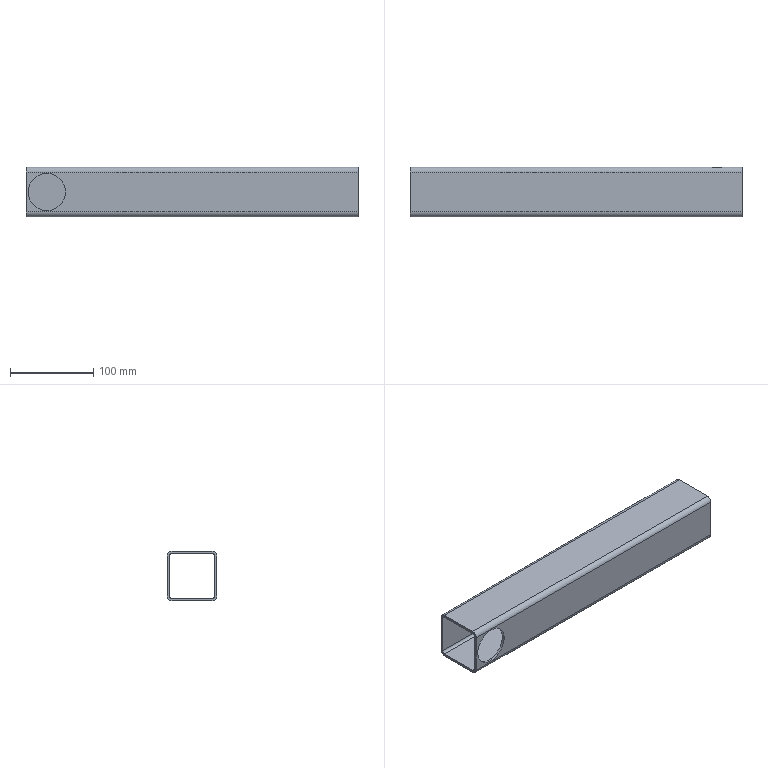Part | STEP file | JBJ-P-1016-02_Default<As Machined> | 1 solid | 24 faces | box 400 x 60 x 60 mm | volume 252664 mm3 | plane 12 | cylinder 12 | commonest cylinder face diameters 6 x6 12 x4 45 x1 54 x1
STEP:
#1=CARTESIAN_POINT('',(400.,30.,-24.));
#2=VERTEX_POINT('',#1);
#3=CARTESIAN_POINT('',(382.369,30.,-24.));
#4=VERTEX_POINT('',#3);
#5=CARTESIAN_POINT('',(400.,30.,-24.));
#6=DIRECTION('',(-1.,0.,0.));
#7=VECTOR('',#6,1000.);
#8=LINE('',#5,#7);
#9=EDGE_CURVE('',#2,#4,#8,.T.);
#10=ORIENTED_EDGE('',*,*,#9,.T.);
#11=CARTESIAN_POINT('',(382.369,30.,24.));
#12=VERTEX_POINT('',#11);
#13=CARTESIAN_POINT('',(370.,30.,0.));
#14=DIRECTION('',(0.,1.,0.));
#15=DIRECTION('',(0.,0.,1.));
#16=AXIS2_PLACEMENT_3D('',#13,#14,#15);
#17=CIRCLE('',#16,27.);
#18=EDGE_CURVE('',#12,#4,#17,.T.);
#19=ORIENTED_EDGE('',*,*,#18,.F.);
#20=CARTESIAN_POINT('',(400.,30.,24.));
#21=VERTEX_POINT('',#20);
#22=CARTESIAN_POINT('',(400.,30.,24.));
#23=DIRECTION('',(-1.,0.,0.));
#24=VECTOR('',#23,1000.);
#25=LINE('',#22,#24);
#26=EDGE_CURVE('',#21,#12,#25,.T.);
#27=ORIENTED_EDGE('',*,*,#26,.F.);
#28=CARTESIAN_POINT('',(400.,30.,-24.));
#29=DIRECTION('',(0.,0.,1.));
#30=VECTOR('',#29,1000.);
#31=LINE('',#28,#30);
#32=EDGE_CURVE('',#2,#21,#31,.T.);
#33=ORIENTED_EDGE('',*,*,#32,.F.);
#34=EDGE_LOOP('',(#10,#19,#27,#33));
#35=FACE_OUTER_BOUND('',#34,.T.);
#36=CARTESIAN_POINT('',(400.,30.,-24.));
#37=DIRECTION('',(0.,-1.,0.));
#38=DIRECTION('',(0.,0.,-1.));
#39=AXIS2_PLACEMENT_3D('',#36,#37,#38);
#40=PLANE('',#39);
#41=ADVANCED_FACE('',(#35),#40,.F.);
#42=CARTESIAN_POINT('',(370.,24.,27.));
#43=VERTEX_POINT('',#42);
#44=CARTESIAN_POINT('',(382.369,27.,24.));
#45=VERTEX_POINT('',#44);
#46=CARTESIAN_POINT('',(370.,24.,27.));
#47=CARTESIAN_POINT('',(370.261,24.087,27.));
#48=CARTESIAN_POINT('',(370.526,24.175,26.996));
#49=CARTESIAN_POINT('',(371.05,24.35,26.981));
#50=CARTESIAN_POINT('',(371.312,24.436,26.969));
#51=CARTESIAN_POINT('',(372.097,24.695,26.924));
#52=CARTESIAN_POINT('',(372.618,24.866,26.878));
#53=CARTESIAN_POINT('',(374.18,25.364,26.695));
#54=CARTESIAN_POINT('',(375.217,25.682,26.513));
#55=CARTESIAN_POINT('',(376.773,26.109,26.142));
#56=CARTESIAN_POINT('',(377.294,26.243,26.002));
#57=CARTESIAN_POINT('',(378.33,26.488,25.689));
#58=CARTESIAN_POINT('',(378.844,26.597,25.516));
#59=CARTESIAN_POINT('',(379.863,26.783,25.14));
#60=CARTESIAN_POINT('',(380.369,26.859,24.935));
#61=CARTESIAN_POINT('',(381.374,26.968,24.494));
#62=CARTESIAN_POINT('',(381.873,27.,24.256));
#63=CARTESIAN_POINT('',(382.369,27.,24.));
#64=B_SPLINE_CURVE_WITH_KNOTS('',3,(#46,#47,#48,#49,#50,#51,#52,#53,#54,#55,#56,#57,#58,#59,#60,#61,#62,#63),.UNSPECIFIED.,.F.,.F.,(4,2,2,2,2,2,2,2,4),(-0.00003286,0.0007915,0.001616,0.003265,0.006562,0.008211,0.00986,0.01151,0.01316),.UNSPECIFIED.);
#65=EDGE_CURVE('',#43,#45,#64,.T.);
#66=ORIENTED_EDGE('',*,*,#65,.T.);
#67=CARTESIAN_POINT('',(400.,27.,24.));
#68=VERTEX_POINT('',#67);
#69=CARTESIAN_POINT('',(400.,27.,24.));
#70=DIRECTION('',(-1.,0.,0.));
#71=VECTOR('',#70,1000.);
#72=LINE('',#69,#71);
#73=EDGE_CURVE('',#68,#45,#72,.T.);
#74=ORIENTED_EDGE('',*,*,#73,.F.);
#75=CARTESIAN_POINT('',(400.,24.,27.));
#76=VERTEX_POINT('',#75);
#77=CARTESIAN_POINT('',(400.,24.,24.));
#78=DIRECTION('',(1.,0.,0.));
#79=DIRECTION('',(0.,0.,-1.));
#80=AXIS2_PLACEMENT_3D('',#77,#78,#79);
#81=CIRCLE('',#80,3.);
#82=EDGE_CURVE('',#68,#76,#81,.T.);
#83=ORIENTED_EDGE('',*,*,#82,.T.);
#84=CARTESIAN_POINT('',(400.,24.,27.));
#85=DIRECTION('',(-1.,0.,0.));
#86=VECTOR('',#85,1000.);
#87=LINE('',#84,#86);
#88=EDGE_CURVE('',#76,#43,#87,.T.);
#89=ORIENTED_EDGE('',*,*,#88,.T.);
#90=EDGE_LOOP('',(#66,#74,#83,#89));
#91=FACE_OUTER_BOUND('',#90,.T.);
#92=CARTESIAN_POINT('',(400.,24.,24.));
#93=DIRECTION('',(-1.,0.,0.));
#94=DIRECTION('',(0.,0.,1.));
#95=AXIS2_PLACEMENT_3D('',#92,#93,#94);
#96=CYLINDRICAL_SURFACE('',#95,3.);
#97=ADVANCED_FACE('',(#91),#96,.F.);
#98=CARTESIAN_POINT('',(382.369,27.,-24.));
#99=VERTEX_POINT('',#98);
#100=CARTESIAN_POINT('',(370.,27.,0.));
#101=DIRECTION('',(0.,1.,0.));
#102=DIRECTION('',(0.,0.,-1.));
#103=AXIS2_PLACEMENT_3D('',#100,#101,#102);
#104=CIRCLE('',#103,27.);
#105=EDGE_CURVE('',#45,#99,#104,.T.);
#106=ORIENTED_EDGE('',*,*,#105,.T.);
#107=CARTESIAN_POINT('',(400.,27.,-24.));
#108=VERTEX_POINT('',#107);
#109=CARTESIAN_POINT('',(400.,27.,-24.));
#110=DIRECTION('',(-1.,0.,0.));
#111=VECTOR('',#110,1000.);
#112=LINE('',#109,#111);
#113=EDGE_CURVE('',#108,#99,#112,.T.);
#114=ORIENTED_EDGE('',*,*,#113,.F.);
#115=CARTESIAN_POINT('',(400.,27.,-24.));
#116=DIRECTION('',(0.,0.,1.));
#117=VECTOR('',#116,1000.);
#118=LINE('',#115,#117);
#119=EDGE_CURVE('',#108,#68,#118,.T.);
#120=ORIENTED_EDGE('',*,*,#119,.T.);
#121=ORIENTED_EDGE('',*,*,#73,.T.);
#122=EDGE_LOOP('',(#106,#114,#120,#121));
#123=FACE_OUTER_BOUND('',#122,.T.);
#124=CARTESIAN_POINT('',(400.,27.,-24.));
#125=DIRECTION('',(0.,-1.,0.));
#126=DIRECTION('',(0.,0.,-1.));
#127=AXIS2_PLACEMENT_3D('',#124,#125,#126);
#128=PLANE('',#127);
#129=ADVANCED_FACE('',(#123),#128,.T.);
#130=CARTESIAN_POINT('',(370.,24.,-27.));
#131=VERTEX_POINT('',#130);
#132=CARTESIAN_POINT('',(357.631,27.,-24.));
#133=VERTEX_POINT('',#132);
#134=CARTESIAN_POINT('',(370.,24.,-27.));
#135=CARTESIAN_POINT('',(369.739,24.087,-27.));
#136=CARTESIAN_POINT('',(369.474,24.175,-26.996));
#137=CARTESIAN_POINT('',(368.95,24.35,-26.981));
#138=CARTESIAN_POINT('',(368.688,24.436,-26.969));
#139=CARTESIAN_POINT('',(367.903,24.695,-26.924));
#140=CARTESIAN_POINT('',(367.382,24.866,-26.878));
#141=CARTESIAN_POINT('',(365.82,25.364,-26.695));
#142=CARTESIAN_POINT('',(364.783,25.682,-26.513));
#143=CARTESIAN_POINT('',(363.227,26.109,-26.142));
#144=CARTESIAN_POINT('',(362.706,26.243,-26.002));
#145=CARTESIAN_POINT('',(361.67,26.488,-25.689));
#146=CARTESIAN_POINT('',(361.156,26.597,-25.516));
#147=CARTESIAN_POINT('',(360.137,26.783,-25.14));
#148=CARTESIAN_POINT('',(359.631,26.859,-24.935));
#149=CARTESIAN_POINT('',(358.626,26.968,-24.494));
#150=CARTESIAN_POINT('',(358.127,27.,-24.256));
#151=CARTESIAN_POINT('',(357.631,27.,-24.));
#152=B_SPLINE_CURVE_WITH_KNOTS('',3,(#134,#135,#136,#137,#138,#139,#140,#141,#142,#143,#144,#145,#146,#147,#148,#149,#150,#151),.UNSPECIFIED.,.F.,.F.,(4,2,2,2,2,2,2,2,4),(-0.00003286,0.0007915,0.001616,0.003265,0.006562,0.008211,0.00986,0.01151,0.01316),.UNSPECIFIED.);
#153=EDGE_CURVE('',#131,#133,#152,.T.);
#154=ORIENTED_EDGE('',*,*,#153,.T.);
#155=CARTESIAN_POINT('',(0.,27.,-24.));
#156=VERTEX_POINT('',#155);
#157=CARTESIAN_POINT('',(400.,27.,-24.));
#158=DIRECTION('',(-1.,0.,0.));
#159=VECTOR('',#158,1000.);
#160=LINE('',#157,#159);
#161=EDGE_CURVE('',#133,#156,#160,.T.);
#162=ORIENTED_EDGE('',*,*,#161,.T.);
#163=CARTESIAN_POINT('',(0.,24.,-27.));
#164=VERTEX_POINT('',#163);
#165=CARTESIAN_POINT('',(0.,24.,-24.));
#166=DIRECTION('',(1.,0.,0.));
#167=DIRECTION('',(0.,0.,-1.));
#168=AXIS2_PLACEMENT_3D('',#165,#166,#167);
#169=CIRCLE('',#168,3.);
#170=EDGE_CURVE('',#164,#156,#169,.T.);
#171=ORIENTED_EDGE('',*,*,#170,.F.);
#172=CARTESIAN_POINT('',(400.,24.,-27.));
#173=DIRECTION('',(-1.,0.,0.));
#174=VECTOR('',#173,1000.);
#175=LINE('',#172,#174);
#176=EDGE_CURVE('',#131,#164,#175,.T.);
#177=ORIENTED_EDGE('',*,*,#176,.F.);
#178=EDGE_LOOP('',(#154,#162,#171,#177));
#179=FACE_OUTER_BOUND('',#178,.T.);
#180=CARTESIAN_POINT('',(400.,24.,-24.));
#181=DIRECTION('',(-1.,0.,0.));
#182=DIRECTION('',(0.,0.,1.));
#183=AXIS2_PLACEMENT_3D('',#180,#181,#182);
#184=CYLINDRICAL_SURFACE('',#183,3.);
#185=ADVANCED_FACE('',(#179),#184,.F.);
#186=CARTESIAN_POINT('',(357.631,30.,-24.));
#187=VERTEX_POINT('',#186);
#188=CARTESIAN_POINT('',(0.,30.,-24.));
#189=VERTEX_POINT('',#188);
#190=CARTESIAN_POINT('',(400.,30.,-24.));
#191=DIRECTION('',(-1.,0.,0.));
#192=VECTOR('',#191,1000.);
#193=LINE('',#190,#192);
#194=EDGE_CURVE('',#187,#189,#193,.T.);
#195=ORIENTED_EDGE('',*,*,#194,.F.);
#196=CARTESIAN_POINT('',(382.369,30.,-24.));
#197=CARTESIAN_POINT('',(381.404,30.,-24.497));
#198=CARTESIAN_POINT('',(380.422,29.94,-24.93));
#199=CARTESIAN_POINT('',(378.422,29.774,-25.675));
#200=CARTESIAN_POINT('',(377.403,29.668,-25.987));
#201=CARTESIAN_POINT('',(375.845,29.516,-26.365));
#202=CARTESIAN_POINT('',(375.32,29.466,-26.476));
#203=CARTESIAN_POINT('',(374.26,29.376,-26.667));
#204=CARTESIAN_POINT('',(373.726,29.335,-26.747));
#205=CARTESIAN_POINT('',(372.13,29.234,-26.937));
#206=CARTESIAN_POINT('',(371.065,29.196,-27.));
#207=CARTESIAN_POINT('',(368.934,29.196,-27.));
#208=CARTESIAN_POINT('',(367.868,29.234,-26.937));
#209=CARTESIAN_POINT('',(366.267,29.335,-26.746));
#210=CARTESIAN_POINT('',(365.732,29.376,-26.666));
#211=CARTESIAN_POINT('',(364.674,29.467,-26.475));
#212=CARTESIAN_POINT('',(364.15,29.516,-26.364));
#213=CARTESIAN_POINT('',(362.594,29.668,-25.986));
#214=CARTESIAN_POINT('',(361.577,29.774,-25.675));
#215=CARTESIAN_POINT('',(359.578,29.94,-24.93));
#216=CARTESIAN_POINT('',(358.596,30.,-24.497));
#217=CARTESIAN_POINT('',(357.631,30.,-24.));
#218=B_SPLINE_CURVE_WITH_KNOTS('',3,(#196,#197,#198,#199,#200,#201,#202,#203,#204,#205,#206,#207,#208,#209,#210,#211,#212,#213,#214,#215,#216,#217),.UNSPECIFIED.,.F.,.F.,(4,2,2,2,2,2,2,2,2,2,4),(0.,0.00321,0.00642,0.008025,0.00963,0.01284,0.01605,0.01765,0.01926,0.02247,0.02568),.UNSPECIFIED.);
#219=EDGE_CURVE('',#4,#187,#218,.T.);
#220=ORIENTED_EDGE('',*,*,#219,.F.);
#221=ORIENTED_EDGE('',*,*,#9,.F.);
#222=CARTESIAN_POINT('',(400.,24.,-30.));
#223=VERTEX_POINT('',#222);
#224=CARTESIAN_POINT('',(400.,24.,-24.));
#225=DIRECTION('',(1.,0.,0.));
#226=DIRECTION('',(0.,0.,-1.));
#227=AXIS2_PLACEMENT_3D('',#224,#225,#226);
#228=CIRCLE('',#227,6.);
#229=EDGE_CURVE('',#223,#2,#228,.T.);
#230=ORIENTED_EDGE('',*,*,#229,.F.);
#231=CARTESIAN_POINT('',(0.,24.,-30.));
#232=VERTEX_POINT('',#231);
#233=CARTESIAN_POINT('',(400.,24.,-30.));
#234=DIRECTION('',(-1.,0.,0.));
#235=VECTOR('',#234,1000.);
#236=LINE('',#233,#235);
#237=EDGE_CURVE('',#223,#232,#236,.T.);
#238=ORIENTED_EDGE('',*,*,#237,.T.);
#239=CARTESIAN_POINT('',(0.,24.,-24.));
#240=DIRECTION('',(1.,0.,0.));
#241=DIRECTION('',(0.,0.,-1.));
#242=AXIS2_PLACEMENT_3D('',#239,#240,#241);
#243=CIRCLE('',#242,6.);
#244=EDGE_CURVE('',#232,#189,#243,.T.);
#245=ORIENTED_EDGE('',*,*,#244,.T.);
#246=EDGE_LOOP('',(#195,#220,#221,#230,#238,#245));
#247=FACE_OUTER_BOUND('',#246,.T.);
#248=CARTESIAN_POINT('',(400.,24.,-24.));
#249=DIRECTION('',(-1.,0.,0.));
#250=DIRECTION('',(0.,0.,1.));
#251=AXIS2_PLACEMENT_3D('',#248,#249,#250);
#252=CYLINDRICAL_SURFACE('',#251,6.);
#253=ADVANCED_FACE('',(#247),#252,.T.);
#254=CARTESIAN_POINT('',(357.631,30.,24.));
#255=VERTEX_POINT('',#254);
#256=CARTESIAN_POINT('',(0.,30.,24.));
#257=VERTEX_POINT('',#256);
#258=CARTESIAN_POINT('',(400.,30.,24.));
#259=DIRECTION('',(-1.,0.,0.));
#260=VECTOR('',#259,1000.);
#261=LINE('',#258,#260);
#262=EDGE_CURVE('',#255,#257,#261,.T.);
#263=ORIENTED_EDGE('',*,*,#262,.F.);
#264=CARTESIAN_POINT('',(370.,30.,0.));
#265=DIRECTION('',(0.,1.,0.));
#266=DIRECTION('',(0.,0.,1.));
#267=AXIS2_PLACEMENT_3D('',#264,#265,#266);
#268=CIRCLE('',#267,27.);
#269=EDGE_CURVE('',#187,#255,#268,.T.);
#270=ORIENTED_EDGE('',*,*,#269,.F.);
#271=ORIENTED_EDGE('',*,*,#194,.T.);
#272=CARTESIAN_POINT('',(0.,30.,-24.));
#273=DIRECTION('',(0.,0.,1.));
#274=VECTOR('',#273,1000.);
#275=LINE('',#272,#274);
#276=EDGE_CURVE('',#189,#257,#275,.T.);
#277=ORIENTED_EDGE('',*,*,#276,.T.);
#278=EDGE_LOOP('',(#263,#270,#271,#277));
#279=FACE_OUTER_BOUND('',#278,.T.);
#280=CARTESIAN_POINT('',(400.,30.,-24.));
#281=DIRECTION('',(0.,-1.,0.));
#282=DIRECTION('',(0.,0.,-1.));
#283=AXIS2_PLACEMENT_3D('',#280,#281,#282);
#284=PLANE('',#283);
#285=ADVANCED_FACE('',(#279),#284,.F.);
#286=ORIENTED_EDGE('',*,*,#26,.T.);
#287=CARTESIAN_POINT('',(357.631,30.,24.));
#288=CARTESIAN_POINT('',(358.596,30.,24.497));
#289=CARTESIAN_POINT('',(359.578,29.94,24.93));
#290=CARTESIAN_POINT('',(361.578,29.774,25.675));
#291=CARTESIAN_POINT('',(362.597,29.668,25.987));
#292=CARTESIAN_POINT('',(364.155,29.516,26.365));
#293=CARTESIAN_POINT('',(364.68,29.466,26.476));
#294=CARTESIAN_POINT('',(365.74,29.376,26.667));
#295=CARTESIAN_POINT('',(366.274,29.335,26.747));
#296=CARTESIAN_POINT('',(367.87,29.234,26.937));
#297=CARTESIAN_POINT('',(368.935,29.196,27.));
#298=CARTESIAN_POINT('',(371.066,29.196,27.));
#299=CARTESIAN_POINT('',(372.132,29.234,26.937));
#300=CARTESIAN_POINT('',(373.733,29.335,26.746));
#301=CARTESIAN_POINT('',(374.268,29.376,26.666));
#302=CARTESIAN_POINT('',(375.326,29.467,26.475));
#303=CARTESIAN_POINT('',(375.85,29.516,26.364));
#304=CARTESIAN_POINT('',(377.406,29.668,25.986));
#305=CARTESIAN_POINT('',(378.423,29.774,25.675));
#306=CARTESIAN_POINT('',(380.422,29.94,24.93));
#307=CARTESIAN_POINT('',(381.404,30.,24.497));
#308=CARTESIAN_POINT('',(382.369,30.,24.));
#309=B_SPLINE_CURVE_WITH_KNOTS('',3,(#287,#288,#289,#290,#291,#292,#293,#294,#295,#296,#297,#298,#299,#300,#301,#302,#303,#304,#305,#306,#307,#308),.UNSPECIFIED.,.F.,.F.,(4,2,2,2,2,2,2,2,2,2,4),(0.,0.00321,0.00642,0.008025,0.00963,0.01284,0.01605,0.01765,0.01926,0.02247,0.02568),.UNSPECIFIED.);
#310=EDGE_CURVE('',#255,#12,#309,.T.);
#311=ORIENTED_EDGE('',*,*,#310,.F.);
#312=ORIENTED_EDGE('',*,*,#262,.T.);
#313=CARTESIAN_POINT('',(0.,24.,30.));
#314=VERTEX_POINT('',#313);
#315=CARTESIAN_POINT('',(0.,24.,24.));
#316=DIRECTION('',(1.,0.,0.));
#317=DIRECTION('',(0.,0.,-1.));
#318=AXIS2_PLACEMENT_3D('',#315,#316,#317);
#319=CIRCLE('',#318,6.);
#320=EDGE_CURVE('',#257,#314,#319,.T.);
#321=ORIENTED_EDGE('',*,*,#320,.T.);
#322=CARTESIAN_POINT('',(400.,24.,30.));
#323=VERTEX_POINT('',#322);
#324=CARTESIAN_POINT('',(400.,24.,30.));
#325=DIRECTION('',(-1.,0.,0.));
#326=VECTOR('',#325,1000.);
#327=LINE('',#324,#326);
#328=EDGE_CURVE('',#323,#314,#327,.T.);
#329=ORIENTED_EDGE('',*,*,#328,.F.);
#330=CARTESIAN_POINT('',(400.,24.,24.));
#331=DIRECTION('',(1.,0.,0.));
#332=DIRECTION('',(0.,0.,-1.));
#333=AXIS2_PLACEMENT_3D('',#330,#331,#332);
#334=CIRCLE('',#333,6.);
#335=EDGE_CURVE('',#21,#323,#334,.T.);
#336=ORIENTED_EDGE('',*,*,#335,.F.);
#337=EDGE_LOOP('',(#286,#311,#312,#321,#329,#336));
#338=FACE_OUTER_BOUND('',#337,.T.);
#339=CARTESIAN_POINT('',(400.,24.,24.));
#340=DIRECTION('',(-1.,0.,0.));
#341=DIRECTION('',(0.,0.,1.));
#342=AXIS2_PLACEMENT_3D('',#339,#340,#341);
#343=CYLINDRICAL_SURFACE('',#342,6.);
#344=ADVANCED_FACE('',(#338),#343,.T.);
#345=CARTESIAN_POINT('',(0.,-24.,30.));
#346=VERTEX_POINT('',#345);
#347=CARTESIAN_POINT('',(0.,-24.,30.));
#348=DIRECTION('',(0.,-1.,0.));
#349=VECTOR('',#348,1000.);
#350=LINE('',#347,#349);
#351=EDGE_CURVE('',#314,#346,#350,.T.);
#352=ORIENTED_EDGE('',*,*,#351,.T.);
#353=CARTESIAN_POINT('',(400.,-24.,30.));
#354=VERTEX_POINT('',#353);
#355=CARTESIAN_POINT('',(400.,-24.,30.));
#356=DIRECTION('',(-1.,0.,0.));
#357=VECTOR('',#356,1000.);
#358=LINE('',#355,#357);
#359=EDGE_CURVE('',#354,#346,#358,.T.);
#360=ORIENTED_EDGE('',*,*,#359,.F.);
#361=CARTESIAN_POINT('',(400.,-24.,30.));
#362=DIRECTION('',(0.,-1.,0.));
#363=VECTOR('',#362,1000.);
#364=LINE('',#361,#363);
#365=EDGE_CURVE('',#323,#354,#364,.T.);
#366=ORIENTED_EDGE('',*,*,#365,.F.);
#367=ORIENTED_EDGE('',*,*,#328,.T.);
#368=EDGE_LOOP('',(#352,#360,#366,#367));
#369=FACE_OUTER_BOUND('',#368,.T.);
#370=CARTESIAN_POINT('',(400.,-24.,30.));
#371=DIRECTION('',(0.,0.,-1.));
#372=DIRECTION('',(-1.,0.,0.));
#373=AXIS2_PLACEMENT_3D('',#370,#371,#372);
#374=PLANE('',#373);
#375=ADVANCED_FACE('',(#369),#374,.F.);
#376=CARTESIAN_POINT('',(0.,-30.,24.));
#377=VERTEX_POINT('',#376);
#378=CARTESIAN_POINT('',(0.,-24.,24.));
#379=DIRECTION('',(1.,0.,0.));
#380=DIRECTION('',(0.,0.,-1.));
#381=AXIS2_PLACEMENT_3D('',#378,#379,#380);
#382=CIRCLE('',#381,6.);
#383=EDGE_CURVE('',#346,#377,#382,.T.);
#384=ORIENTED_EDGE('',*,*,#383,.T.);
#385=CARTESIAN_POINT('',(400.,-30.,24.));
#386=VERTEX_POINT('',#385);
#387=CARTESIAN_POINT('',(400.,-30.,24.));
#388=DIRECTION('',(-1.,0.,0.));
#389=VECTOR('',#388,1000.);
#390=LINE('',#387,#389);
#391=EDGE_CURVE('',#386,#377,#390,.T.);
#392=ORIENTED_EDGE('',*,*,#391,.F.);
#393=CARTESIAN_POINT('',(400.,-24.,24.));
#394=DIRECTION('',(1.,0.,0.));
#395=DIRECTION('',(0.,0.,-1.));
#396=AXIS2_PLACEMENT_3D('',#393,#394,#395);
#397=CIRCLE('',#396,6.);
#398=EDGE_CURVE('',#354,#386,#397,.T.);
#399=ORIENTED_EDGE('',*,*,#398,.F.);
#400=ORIENTED_EDGE('',*,*,#359,.T.);
#401=EDGE_LOOP('',(#384,#392,#399,#400));
#402=FACE_OUTER_BOUND('',#401,.T.);
#403=CARTESIAN_POINT('',(400.,-24.,24.));
#404=DIRECTION('',(-1.,0.,0.));
#405=DIRECTION('',(0.,0.,1.));
#406=AXIS2_PLACEMENT_3D('',#403,#404,#405);
#407=CYLINDRICAL_SURFACE('',#406,6.);
#408=ADVANCED_FACE('',(#402),#407,.T.);
#409=CARTESIAN_POINT('',(25.,-30.,-22.5));
#410=VERTEX_POINT('',#409);
#411=CARTESIAN_POINT('',(25.,-30.,0.));
#412=DIRECTION('',(0.,-1.,0.));
#413=DIRECTION('',(0.,0.,-1.));
#414=AXIS2_PLACEMENT_3D('',#411,#412,#413);
#415=CIRCLE('',#414,22.5);
#416=EDGE_CURVE('',#410,#410,#415,.T.);
#417=ORIENTED_EDGE('',*,*,#416,.F.);
#418=EDGE_LOOP('',(#417));
#419=FACE_BOUND('',#418,.T.);
#420=CARTESIAN_POINT('',(0.,-30.,-24.));
#421=VERTEX_POINT('',#420);
#422=CARTESIAN_POINT('',(0.,-30.,24.));
#423=DIRECTION('',(0.,0.,-1.));
#424=VECTOR('',#423,1000.);
#425=LINE('',#422,#424);
#426=EDGE_CURVE('',#377,#421,#425,.T.);
#427=ORIENTED_EDGE('',*,*,#426,.T.);
#428=CARTESIAN_POINT('',(400.,-30.,-24.));
#429=VERTEX_POINT('',#428);
#430=CARTESIAN_POINT('',(400.,-30.,-24.));
#431=DIRECTION('',(-1.,0.,0.));
#432=VECTOR('',#431,1000.);
#433=LINE('',#430,#432);
#434=EDGE_CURVE('',#429,#421,#433,.T.);
#435=ORIENTED_EDGE('',*,*,#434,.F.);
#436=CARTESIAN_POINT('',(400.,-30.,24.));
#437=DIRECTION('',(0.,0.,-1.));
#438=VECTOR('',#437,1000.);
#439=LINE('',#436,#438);
#440=EDGE_CURVE('',#386,#429,#439,.T.);
#441=ORIENTED_EDGE('',*,*,#440,.F.);
#442=ORIENTED_EDGE('',*,*,#391,.T.);
#443=EDGE_LOOP('',(#427,#435,#441,#442));
#444=FACE_OUTER_BOUND('',#443,.T.);
#445=CARTESIAN_POINT('',(400.,-30.,24.));
#446=DIRECTION('',(0.,1.,0.));
#447=DIRECTION('',(0.,0.,1.));
#448=AXIS2_PLACEMENT_3D('',#445,#446,#447);
#449=PLANE('',#448);
#450=ADVANCED_FACE('',(#419,#444),#449,.F.);
#451=CARTESIAN_POINT('',(0.,-24.,-30.));
#452=VERTEX_POINT('',#451);
#453=CARTESIAN_POINT('',(0.,-24.,-24.));
#454=DIRECTION('',(1.,0.,0.));
#455=DIRECTION('',(0.,0.,-1.));
#456=AXIS2_PLACEMENT_3D('',#453,#454,#455);
#457=CIRCLE('',#456,6.);
#458=EDGE_CURVE('',#421,#452,#457,.T.);
#459=ORIENTED_EDGE('',*,*,#458,.T.);
#460=CARTESIAN_POINT('',(400.,-24.,-30.));
#461=VERTEX_POINT('',#460);
#462=CARTESIAN_POINT('',(400.,-24.,-30.));
#463=DIRECTION('',(-1.,0.,0.));
#464=VECTOR('',#463,1000.);
#465=LINE('',#462,#464);
#466=EDGE_CURVE('',#461,#452,#465,.T.);
#467=ORIENTED_EDGE('',*,*,#466,.F.);
#468=CARTESIAN_POINT('',(400.,-24.,-24.));
#469=DIRECTION('',(1.,0.,0.));
#470=DIRECTION('',(0.,0.,-1.));
#471=AXIS2_PLACEMENT_3D('',#468,#469,#470);
#472=CIRCLE('',#471,6.);
#473=EDGE_CURVE('',#429,#461,#472,.T.);
#474=ORIENTED_EDGE('',*,*,#473,.F.);
#475=ORIENTED_EDGE('',*,*,#434,.T.);
#476=EDGE_LOOP('',(#459,#467,#474,#475));
#477=FACE_OUTER_BOUND('',#476,.T.);
#478=CARTESIAN_POINT('',(400.,-24.,-24.));
#479=DIRECTION('',(-1.,0.,0.));
#480=DIRECTION('',(0.,0.,1.));
#481=AXIS2_PLACEMENT_3D('',#478,#479,#480);
#482=CYLINDRICAL_SURFACE('',#481,6.);
#483=ADVANCED_FACE('',(#477),#482,.T.);
#484=CARTESIAN_POINT('',(357.631,27.,24.));
#485=VERTEX_POINT('',#484);
#486=CARTESIAN_POINT('',(357.631,27.,24.));
#487=CARTESIAN_POINT('',(358.127,27.,24.256));
#488=CARTESIAN_POINT('',(358.626,26.968,24.494));
#489=CARTESIAN_POINT('',(359.631,26.859,24.935));
#490=CARTESIAN_POINT('',(360.137,26.783,25.14));
#491=CARTESIAN_POINT('',(361.156,26.597,25.516));
#492=CARTESIAN_POINT('',(361.67,26.488,25.689));
#493=CARTESIAN_POINT('',(362.706,26.243,26.002));
#494=CARTESIAN_POINT('',(363.227,26.109,26.142));
#495=CARTESIAN_POINT('',(364.783,25.682,26.513));
#496=CARTESIAN_POINT('',(365.82,25.364,26.695));
#497=CARTESIAN_POINT('',(367.382,24.866,26.878));
#498=CARTESIAN_POINT('',(367.903,24.695,26.924));
#499=CARTESIAN_POINT('',(368.688,24.436,26.969));
#500=CARTESIAN_POINT('',(368.95,24.35,26.981));
#501=CARTESIAN_POINT('',(369.474,24.175,26.996));
#502=CARTESIAN_POINT('',(369.739,24.087,27.));
#503=CARTESIAN_POINT('',(370.,24.,27.));
#504=B_SPLINE_CURVE_WITH_KNOTS('',3,(#486,#487,#488,#489,#490,#491,#492,#493,#494,#495,#496,#497,#498,#499,#500,#501,#502,#503),.UNSPECIFIED.,.F.,.F.,(4,2,2,2,2,2,2,2,4),(0.,0.001653,0.003305,0.004958,0.00661,0.009915,0.01157,0.01239,0.01322),.UNSPECIFIED.);
#505=EDGE_CURVE('',#485,#43,#504,.T.);
#506=ORIENTED_EDGE('',*,*,#505,.T.);
#507=CARTESIAN_POINT('',(0.,24.,27.));
#508=VERTEX_POINT('',#507);
#509=CARTESIAN_POINT('',(400.,24.,27.));
#510=DIRECTION('',(-1.,0.,0.));
#511=VECTOR('',#510,1000.);
#512=LINE('',#509,#511);
#513=EDGE_CURVE('',#43,#508,#512,.T.);
#514=ORIENTED_EDGE('',*,*,#513,.T.);
#515=CARTESIAN_POINT('',(0.,27.,24.));
#516=VERTEX_POINT('',#515);
#517=CARTESIAN_POINT('',(0.,24.,24.));
#518=DIRECTION('',(1.,0.,0.));
#519=DIRECTION('',(0.,0.,-1.));
#520=AXIS2_PLACEMENT_3D('',#517,#518,#519);
#521=CIRCLE('',#520,3.);
#522=EDGE_CURVE('',#516,#508,#521,.T.);
#523=ORIENTED_EDGE('',*,*,#522,.F.);
#524=CARTESIAN_POINT('',(400.,27.,24.));
#525=DIRECTION('',(-1.,0.,0.));
#526=VECTOR('',#525,1000.);
#527=LINE('',#524,#526);
#528=EDGE_CURVE('',#485,#516,#527,.T.);
#529=ORIENTED_EDGE('',*,*,#528,.F.);
#530=EDGE_LOOP('',(#506,#514,#523,#529));
#531=FACE_OUTER_BOUND('',#530,.T.);
#532=CARTESIAN_POINT('',(400.,24.,24.));
#533=DIRECTION('',(-1.,0.,0.));
#534=DIRECTION('',(0.,0.,1.));
#535=AXIS2_PLACEMENT_3D('',#532,#533,#534);
#536=CYLINDRICAL_SURFACE('',#535,3.);
#537=ADVANCED_FACE('',(#531),#536,.F.);
#538=CARTESIAN_POINT('',(370.,27.,0.));
#539=DIRECTION('',(0.,1.,0.));
#540=DIRECTION('',(0.,0.,-1.));
#541=AXIS2_PLACEMENT_3D('',#538,#539,#540);
#542=CIRCLE('',#541,27.);
#543=EDGE_CURVE('',#133,#485,#542,.T.);
#544=ORIENTED_EDGE('',*,*,#543,.T.);
#545=ORIENTED_EDGE('',*,*,#528,.T.);
#546=CARTESIAN_POINT('',(0.,27.,-24.));
#547=DIRECTION('',(0.,0.,1.));
#548=VECTOR('',#547,1000.);
#549=LINE('',#546,#548);
#550=EDGE_CURVE('',#156,#516,#549,.T.);
#551=ORIENTED_EDGE('',*,*,#550,.F.);
#552=ORIENTED_EDGE('',*,*,#161,.F.);
#553=EDGE_LOOP('',(#544,#545,#551,#552));
#554=FACE_OUTER_BOUND('',#553,.T.);
#555=CARTESIAN_POINT('',(400.,27.,-24.));
#556=DIRECTION('',(0.,-1.,0.));
#557=DIRECTION('',(0.,0.,-1.));
#558=AXIS2_PLACEMENT_3D('',#555,#556,#557);
#559=PLANE('',#558);
#560=ADVANCED_FACE('',(#554),#559,.T.);
#561=CARTESIAN_POINT('',(382.369,27.,-24.));
#562=CARTESIAN_POINT('',(381.873,27.,-24.256));
#563=CARTESIAN_POINT('',(381.374,26.968,-24.494));
#564=CARTESIAN_POINT('',(380.369,26.859,-24.935));
#565=CARTESIAN_POINT('',(379.863,26.783,-25.14));
#566=CARTESIAN_POINT('',(378.844,26.597,-25.516));
#567=CARTESIAN_POINT('',(378.33,26.488,-25.689));
#568=CARTESIAN_POINT('',(377.294,26.243,-26.002));
#569=CARTESIAN_POINT('',(376.773,26.109,-26.142));
#570=CARTESIAN_POINT('',(375.217,25.682,-26.513));
#571=CARTESIAN_POINT('',(374.18,25.364,-26.695));
#572=CARTESIAN_POINT('',(372.618,24.866,-26.878));
#573=CARTESIAN_POINT('',(372.097,24.695,-26.924));
#574=CARTESIAN_POINT('',(371.312,24.436,-26.969));
#575=CARTESIAN_POINT('',(371.05,24.35,-26.981));
#576=CARTESIAN_POINT('',(370.526,24.175,-26.996));
#577=CARTESIAN_POINT('',(370.261,24.087,-27.));
#578=CARTESIAN_POINT('',(370.,24.,-27.));
#579=B_SPLINE_CURVE_WITH_KNOTS('',3,(#561,#562,#563,#564,#565,#566,#567,#568,#569,#570,#571,#572,#573,#574,#575,#576,#577,#578),.UNSPECIFIED.,.F.,.F.,(4,2,2,2,2,2,2,2,4),(0.,0.001653,0.003305,0.004958,0.00661,0.009915,0.01157,0.01239,0.01322),.UNSPECIFIED.);
#580=EDGE_CURVE('',#99,#131,#579,.T.);
#581=ORIENTED_EDGE('',*,*,#580,.T.);
#582=CARTESIAN_POINT('',(400.,24.,-27.));
#583=VERTEX_POINT('',#582);
#584=CARTESIAN_POINT('',(400.,24.,-27.));
#585=DIRECTION('',(-1.,0.,0.));
#586=VECTOR('',#585,1000.);
#587=LINE('',#584,#586);
#588=EDGE_CURVE('',#583,#131,#587,.T.);
#589=ORIENTED_EDGE('',*,*,#588,.F.);
#590=CARTESIAN_POINT('',(400.,24.,-24.));
#591=DIRECTION('',(1.,0.,0.));
#592=DIRECTION('',(0.,0.,-1.));
#593=AXIS2_PLACEMENT_3D('',#590,#591,#592);
#594=CIRCLE('',#593,3.);
#595=EDGE_CURVE('',#583,#108,#594,.T.);
#596=ORIENTED_EDGE('',*,*,#595,.T.);
#597=ORIENTED_EDGE('',*,*,#113,.T.);
#598=EDGE_LOOP('',(#581,#589,#596,#597));
#599=FACE_OUTER_BOUND('',#598,.T.);
#600=CARTESIAN_POINT('',(400.,24.,-24.));
#601=DIRECTION('',(-1.,0.,0.));
#602=DIRECTION('',(0.,0.,1.));
#603=AXIS2_PLACEMENT_3D('',#600,#601,#602);
#604=CYLINDRICAL_SURFACE('',#603,3.);
#605=ADVANCED_FACE('',(#599),#604,.F.);
#606=CARTESIAN_POINT('',(0.,-24.,-27.));
#607=VERTEX_POINT('',#606);
#608=CARTESIAN_POINT('',(0.,24.,-27.));
#609=DIRECTION('',(0.,1.,0.));
#610=VECTOR('',#609,1000.);
#611=LINE('',#608,#610);
#612=EDGE_CURVE('',#607,#164,#611,.T.);
#613=ORIENTED_EDGE('',*,*,#612,.F.);
#614=CARTESIAN_POINT('',(400.,-24.,-27.));
#615=VERTEX_POINT('',#614);
#616=CARTESIAN_POINT('',(400.,-24.,-27.));
#617=DIRECTION('',(-1.,0.,0.));
#618=VECTOR('',#617,1000.);
#619=LINE('',#616,#618);
#620=EDGE_CURVE('',#615,#607,#619,.T.);
#621=ORIENTED_EDGE('',*,*,#620,.F.);
#622=CARTESIAN_POINT('',(400.,24.,-27.));
#623=DIRECTION('',(0.,1.,0.));
#624=VECTOR('',#623,1000.);
#625=LINE('',#622,#624);
#626=EDGE_CURVE('',#615,#583,#625,.T.);
#627=ORIENTED_EDGE('',*,*,#626,.T.);
#628=ORIENTED_EDGE('',*,*,#588,.T.);
#629=ORIENTED_EDGE('',*,*,#176,.T.);
#630=EDGE_LOOP('',(#613,#621,#627,#628,#629));
#631=FACE_OUTER_BOUND('',#630,.T.);
#632=CARTESIAN_POINT('',(400.,24.,-27.));
#633=DIRECTION('',(0.,0.,1.));
#634=DIRECTION('',(1.,0.,0.));
#635=AXIS2_PLACEMENT_3D('',#632,#633,#634);
#636=PLANE('',#635);
#637=ADVANCED_FACE('',(#631),#636,.T.);
#638=CARTESIAN_POINT('',(0.,-27.,-24.));
#639=VERTEX_POINT('',#638);
#640=CARTESIAN_POINT('',(0.,-24.,-24.));
#641=DIRECTION('',(1.,0.,0.));
#642=DIRECTION('',(0.,0.,-1.));
#643=AXIS2_PLACEMENT_3D('',#640,#641,#642);
#644=CIRCLE('',#643,3.);
#645=EDGE_CURVE('',#639,#607,#644,.T.);
#646=ORIENTED_EDGE('',*,*,#645,.F.);
#647=CARTESIAN_POINT('',(400.,-27.,-24.));
#648=VERTEX_POINT('',#647);
#649=CARTESIAN_POINT('',(400.,-27.,-24.));
#650=DIRECTION('',(-1.,0.,0.));
#651=VECTOR('',#650,1000.);
#652=LINE('',#649,#651);
#653=EDGE_CURVE('',#648,#639,#652,.T.);
#654=ORIENTED_EDGE('',*,*,#653,.F.);
#655=CARTESIAN_POINT('',(400.,-24.,-24.));
#656=DIRECTION('',(1.,0.,0.));
#657=DIRECTION('',(0.,0.,-1.));
#658=AXIS2_PLACEMENT_3D('',#655,#656,#657);
#659=CIRCLE('',#658,3.);
#660=EDGE_CURVE('',#648,#615,#659,.T.);
#661=ORIENTED_EDGE('',*,*,#660,.T.);
#662=ORIENTED_EDGE('',*,*,#620,.T.);
#663=EDGE_LOOP('',(#646,#654,#661,#662));
#664=FACE_OUTER_BOUND('',#663,.T.);
#665=CARTESIAN_POINT('',(400.,-24.,-24.));
#666=DIRECTION('',(-1.,0.,0.));
#667=DIRECTION('',(0.,0.,1.));
#668=AXIS2_PLACEMENT_3D('',#665,#666,#667);
#669=CYLINDRICAL_SURFACE('',#668,3.);
#670=ADVANCED_FACE('',(#664),#669,.F.);
#671=CARTESIAN_POINT('',(25.,-27.,22.5));
#672=VERTEX_POINT('',#671);
#673=CARTESIAN_POINT('',(25.,-27.,0.));
#674=DIRECTION('',(0.,-1.,0.));
#675=DIRECTION('',(0.,0.,1.));
#676=AXIS2_PLACEMENT_3D('',#673,#674,#675);
#677=CIRCLE('',#676,22.5);
#678=EDGE_CURVE('',#672,#672,#677,.T.);
#679=ORIENTED_EDGE('',*,*,#678,.T.);
#680=EDGE_LOOP('',(#679));
#681=FACE_BOUND('',#680,.T.);
#682=CARTESIAN_POINT('',(0.,-27.,24.));
#683=VERTEX_POINT('',#682);
#684=CARTESIAN_POINT('',(0.,-27.,24.));
#685=DIRECTION('',(0.,0.,-1.));
#686=VECTOR('',#685,1000.);
#687=LINE('',#684,#686);
#688=EDGE_CURVE('',#683,#639,#687,.T.);
#689=ORIENTED_EDGE('',*,*,#688,.F.);
#690=CARTESIAN_POINT('',(400.,-27.,24.));
#691=VERTEX_POINT('',#690);
#692=CARTESIAN_POINT('',(400.,-27.,24.));
#693=DIRECTION('',(-1.,0.,0.));
#694=VECTOR('',#693,1000.);
#695=LINE('',#692,#694);
#696=EDGE_CURVE('',#691,#683,#695,.T.);
#697=ORIENTED_EDGE('',*,*,#696,.F.);
#698=CARTESIAN_POINT('',(400.,-27.,24.));
#699=DIRECTION('',(0.,0.,-1.));
#700=VECTOR('',#699,1000.);
#701=LINE('',#698,#700);
#702=EDGE_CURVE('',#691,#648,#701,.T.);
#703=ORIENTED_EDGE('',*,*,#702,.T.);
#704=ORIENTED_EDGE('',*,*,#653,.T.);
#705=EDGE_LOOP('',(#689,#697,#703,#704));
#706=FACE_OUTER_BOUND('',#705,.T.);
#707=CARTESIAN_POINT('',(400.,-27.,24.));
#708=DIRECTION('',(0.,1.,0.));
#709=DIRECTION('',(0.,0.,1.));
#710=AXIS2_PLACEMENT_3D('',#707,#708,#709);
#711=PLANE('',#710);
#712=ADVANCED_FACE('',(#681,#706),#711,.T.);
#713=CARTESIAN_POINT('',(0.,-24.,27.));
#714=VERTEX_POINT('',#713);
#715=CARTESIAN_POINT('',(0.,-24.,24.));
#716=DIRECTION('',(1.,0.,0.));
#717=DIRECTION('',(0.,0.,-1.));
#718=AXIS2_PLACEMENT_3D('',#715,#716,#717);
#719=CIRCLE('',#718,3.);
#720=EDGE_CURVE('',#714,#683,#719,.T.);
#721=ORIENTED_EDGE('',*,*,#720,.F.);
#722=CARTESIAN_POINT('',(400.,-24.,27.));
#723=VERTEX_POINT('',#722);
#724=CARTESIAN_POINT('',(400.,-24.,27.));
#725=DIRECTION('',(-1.,0.,0.));
#726=VECTOR('',#725,1000.);
#727=LINE('',#724,#726);
#728=EDGE_CURVE('',#723,#714,#727,.T.);
#729=ORIENTED_EDGE('',*,*,#728,.F.);
#730=CARTESIAN_POINT('',(400.,-24.,24.));
#731=DIRECTION('',(1.,0.,0.));
#732=DIRECTION('',(0.,0.,-1.));
#733=AXIS2_PLACEMENT_3D('',#730,#731,#732);
#734=CIRCLE('',#733,3.);
#735=EDGE_CURVE('',#723,#691,#734,.T.);
#736=ORIENTED_EDGE('',*,*,#735,.T.);
#737=ORIENTED_EDGE('',*,*,#696,.T.);
#738=EDGE_LOOP('',(#721,#729,#736,#737));
#739=FACE_OUTER_BOUND('',#738,.T.);
#740=CARTESIAN_POINT('',(400.,-24.,24.));
#741=DIRECTION('',(-1.,0.,0.));
#742=DIRECTION('',(0.,0.,1.));
#743=AXIS2_PLACEMENT_3D('',#740,#741,#742);
#744=CYLINDRICAL_SURFACE('',#743,3.);
#745=ADVANCED_FACE('',(#739),#744,.F.);
#746=CARTESIAN_POINT('',(0.,-24.,27.));
#747=DIRECTION('',(0.,-1.,0.));
#748=VECTOR('',#747,1000.);
#749=LINE('',#746,#748);
#750=EDGE_CURVE('',#508,#714,#749,.T.);
#751=ORIENTED_EDGE('',*,*,#750,.F.);
#752=ORIENTED_EDGE('',*,*,#513,.F.);
#753=ORIENTED_EDGE('',*,*,#88,.F.);
#754=CARTESIAN_POINT('',(400.,-24.,27.));
#755=DIRECTION('',(0.,-1.,0.));
#756=VECTOR('',#755,1000.);
#757=LINE('',#754,#756);
#758=EDGE_CURVE('',#76,#723,#757,.T.);
#759=ORIENTED_EDGE('',*,*,#758,.T.);
#760=ORIENTED_EDGE('',*,*,#728,.T.);
#761=EDGE_LOOP('',(#751,#752,#753,#759,#760));
#762=FACE_OUTER_BOUND('',#761,.T.);
#763=CARTESIAN_POINT('',(400.,-24.,27.));
#764=DIRECTION('',(0.,0.,-1.));
#765=DIRECTION('',(-1.,0.,0.));
#766=AXIS2_PLACEMENT_3D('',#763,#764,#765);
#767=PLANE('',#766);
#768=ADVANCED_FACE('',(#762),#767,.T.);
#769=CARTESIAN_POINT('',(0.,24.,-30.));
#770=DIRECTION('',(0.,1.,0.));
#771=VECTOR('',#770,1000.);
#772=LINE('',#769,#771);
#773=EDGE_CURVE('',#452,#232,#772,.T.);
#774=ORIENTED_EDGE('',*,*,#773,.T.);
#775=ORIENTED_EDGE('',*,*,#237,.F.);
#776=CARTESIAN_POINT('',(400.,24.,-30.));
#777=DIRECTION('',(0.,1.,0.));
#778=VECTOR('',#777,1000.);
#779=LINE('',#776,#778);
#780=EDGE_CURVE('',#461,#223,#779,.T.);
#781=ORIENTED_EDGE('',*,*,#780,.F.);
#782=ORIENTED_EDGE('',*,*,#466,.T.);
#783=EDGE_LOOP('',(#774,#775,#781,#782));
#784=FACE_OUTER_BOUND('',#783,.T.);
#785=CARTESIAN_POINT('',(400.,24.,-30.));
#786=DIRECTION('',(0.,0.,1.));
#787=DIRECTION('',(1.,0.,0.));
#788=AXIS2_PLACEMENT_3D('',#785,#786,#787);
#789=PLANE('',#788);
#790=ADVANCED_FACE('',(#784),#789,.F.);
#791=ORIENTED_EDGE('',*,*,#82,.F.);
#792=ORIENTED_EDGE('',*,*,#119,.F.);
#793=ORIENTED_EDGE('',*,*,#595,.F.);
#794=ORIENTED_EDGE('',*,*,#626,.F.);
#795=ORIENTED_EDGE('',*,*,#660,.F.);
#796=ORIENTED_EDGE('',*,*,#702,.F.);
#797=ORIENTED_EDGE('',*,*,#735,.F.);
#798=ORIENTED_EDGE('',*,*,#758,.F.);
#799=EDGE_LOOP('',(#791,#792,#793,#794,#795,#796,#797,#798));
#800=FACE_BOUND('',#799,.T.);
#801=ORIENTED_EDGE('',*,*,#229,.T.);
#802=ORIENTED_EDGE('',*,*,#32,.T.);
#803=ORIENTED_EDGE('',*,*,#335,.T.);
#804=ORIENTED_EDGE('',*,*,#365,.T.);
#805=ORIENTED_EDGE('',*,*,#398,.T.);
#806=ORIENTED_EDGE('',*,*,#440,.T.);
#807=ORIENTED_EDGE('',*,*,#473,.T.);
#808=ORIENTED_EDGE('',*,*,#780,.T.);
#809=EDGE_LOOP('',(#801,#802,#803,#804,#805,#806,#807,#808));
#810=FACE_OUTER_BOUND('',#809,.T.);
#811=CARTESIAN_POINT('',(400.,24.,-24.));
#812=DIRECTION('',(1.,0.,0.));
#813=DIRECTION('',(0.,0.,-1.));
#814=AXIS2_PLACEMENT_3D('',#811,#812,#813);
#815=PLANE('',#814);
#816=ADVANCED_FACE('',(#800,#810),#815,.T.);
#817=ORIENTED_EDGE('',*,*,#522,.T.);
#818=ORIENTED_EDGE('',*,*,#750,.T.);
#819=ORIENTED_EDGE('',*,*,#720,.T.);
#820=ORIENTED_EDGE('',*,*,#688,.T.);
#821=ORIENTED_EDGE('',*,*,#645,.T.);
#822=ORIENTED_EDGE('',*,*,#612,.T.);
#823=ORIENTED_EDGE('',*,*,#170,.T.);
#824=ORIENTED_EDGE('',*,*,#550,.T.);
#825=EDGE_LOOP('',(#817,#818,#819,#820,#821,#822,#823,#824));
#826=FACE_BOUND('',#825,.T.);
#827=ORIENTED_EDGE('',*,*,#244,.F.);
#828=ORIENTED_EDGE('',*,*,#773,.F.);
#829=ORIENTED_EDGE('',*,*,#458,.F.);
#830=ORIENTED_EDGE('',*,*,#426,.F.);
#831=ORIENTED_EDGE('',*,*,#383,.F.);
#832=ORIENTED_EDGE('',*,*,#351,.F.);
#833=ORIENTED_EDGE('',*,*,#320,.F.);
#834=ORIENTED_EDGE('',*,*,#276,.F.);
#835=EDGE_LOOP('',(#827,#828,#829,#830,#831,#832,#833,#834));
#836=FACE_OUTER_BOUND('',#835,.T.);
#837=CARTESIAN_POINT('',(0.,24.,-24.));
#838=DIRECTION('',(1.,0.,0.));
#839=DIRECTION('',(0.,0.,-1.));
#840=AXIS2_PLACEMENT_3D('',#837,#838,#839);
#841=PLANE('',#840);
#842=ADVANCED_FACE('',(#826,#836),#841,.F.);
#843=ORIENTED_EDGE('',*,*,#105,.F.);
#844=ORIENTED_EDGE('',*,*,#65,.F.);
#845=ORIENTED_EDGE('',*,*,#505,.F.);
#846=ORIENTED_EDGE('',*,*,#543,.F.);
#847=ORIENTED_EDGE('',*,*,#153,.F.);
#848=ORIENTED_EDGE('',*,*,#580,.F.);
#849=EDGE_LOOP('',(#843,#844,#845,#846,#847,#848));
#850=FACE_OUTER_BOUND('',#849,.T.);
#851=ORIENTED_EDGE('',*,*,#219,.T.);
#852=ORIENTED_EDGE('',*,*,#269,.T.);
#853=ORIENTED_EDGE('',*,*,#310,.T.);
#854=ORIENTED_EDGE('',*,*,#18,.T.);
#855=EDGE_LOOP('',(#851,#852,#853,#854));
#856=FACE_OUTER_BOUND('',#855,.T.);
#857=CARTESIAN_POINT('',(370.,-30.001,0.));
#858=DIRECTION('',(0.,1.,0.));
#859=DIRECTION('',(0.,0.,1.));
#860=AXIS2_PLACEMENT_3D('',#857,#858,#859);
#861=CYLINDRICAL_SURFACE('',#860,27.);
#862=ADVANCED_FACE('',(#850,#856),#861,.F.);
#863=ORIENTED_EDGE('',*,*,#678,.F.);
#864=EDGE_LOOP('',(#863));
#865=FACE_OUTER_BOUND('',#864,.T.);
#866=ORIENTED_EDGE('',*,*,#416,.T.);
#867=EDGE_LOOP('',(#866));
#868=FACE_OUTER_BOUND('',#867,.T.);
#869=CARTESIAN_POINT('',(25.,30.001,0.));
#870=DIRECTION('',(0.,-1.,0.));
#871=DIRECTION('',(0.,0.,-1.));
#872=AXIS2_PLACEMENT_3D('',#869,#870,#871);
#873=CYLINDRICAL_SURFACE('',#872,22.5);
#874=ADVANCED_FACE('',(#865,#868),#873,.F.);
#875=CLOSED_SHELL('',(#41,#97,#129,#185,#253,#285,#344,#375,#408,#450,#483,#537,#560,#605,#637,#670,#712,#745,#768,#790,#816,#842,#862,#874));
#876=MANIFOLD_SOLID_BREP('',#875);
#877=CARTESIAN_POINT('',(0.,0.,0.));
#878=DIRECTION('',(0.,0.,1.));
#879=DIRECTION('',(1.,0.,0.));
#880=AXIS2_PLACEMENT_3D('',#877,#878,#879);
#881=(LENGTH_UNIT()NAMED_UNIT(*)SI_UNIT(.MILLI.,.METRE.));
#882=UNCERTAINTY_MEASURE_WITH_UNIT(LENGTH_MEASURE(0.00001),#881,'','');
#883=(NAMED_UNIT(*)PLANE_ANGLE_UNIT()SI_UNIT($,.RADIAN.));
#884=(NAMED_UNIT(*)SI_UNIT($,.STERADIAN.)SOLID_ANGLE_UNIT());
#885=(GEOMETRIC_REPRESENTATION_CONTEXT(3)GLOBAL_UNCERTAINTY_ASSIGNED_CONTEXT((#882))GLOBAL_UNIT_ASSIGNED_CONTEXT((#881,#883,#884))REPRESENTATION_CONTEXT('',''));
#886=ADVANCED_BREP_SHAPE_REPRESENTATION('',(#876,#880),#885);